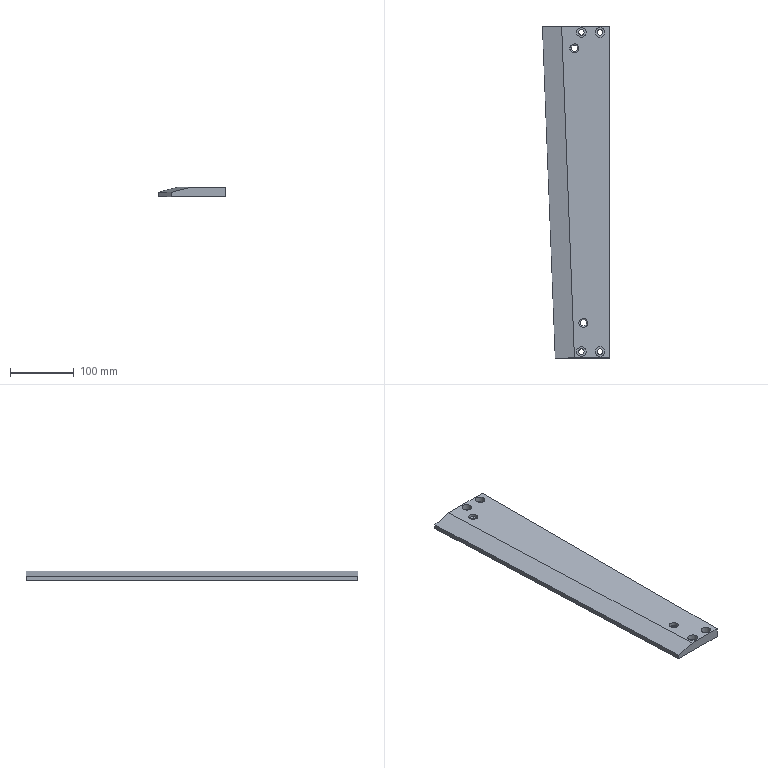Part | STEP file | gslz 2016.10.28-13_id1646_x_t | 1 solid | 25 faces | box 105 x 520 x 15 mm | volume 667550 mm3 | cylinder 12 | plane 11 | cone 2 | commonest cylinder face diameters 8.5 x4 15 x4 10.3 x2 14 x2